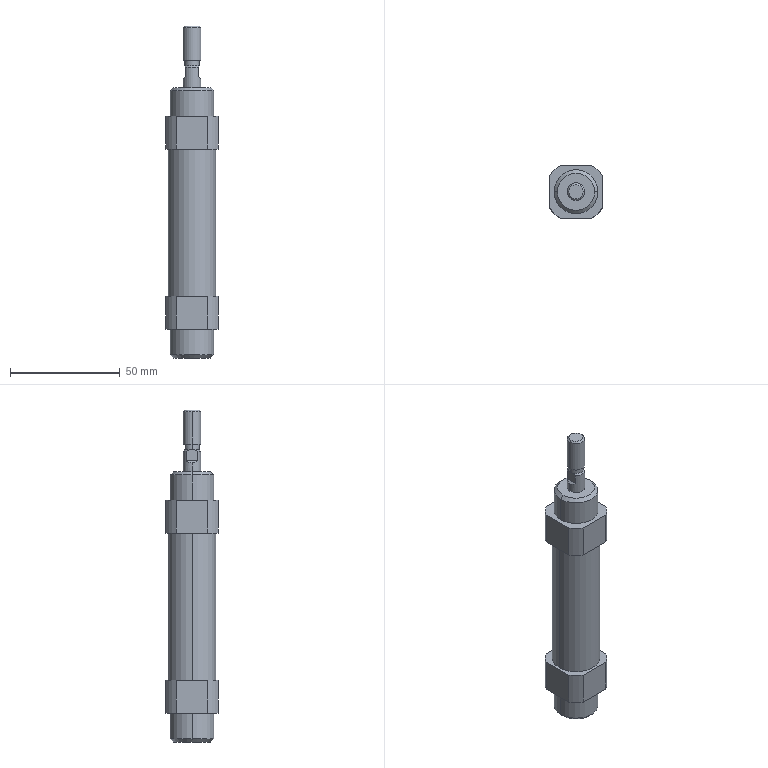Part | STEP file | CDM2B20-35 | 1 solid | 62 faces | box 24 x 24 x 151 mm | volume 48940 mm3 | cylinder 25 | plane 25 | cone 12 | commonest cylinder face diameters 28 x8 8 x5 8.57 x4 20 x4 6.47 x2 21.6 x2